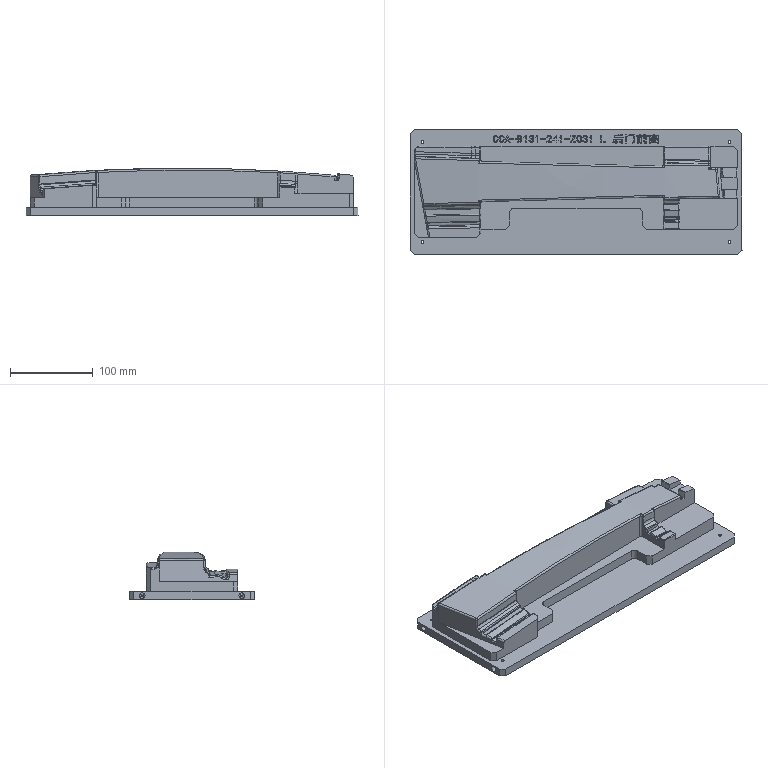NC program | NX | posted with a generic post | part box 400 x 150 x 57.494 mm
Lines 1 to 1105 of 16235:
N10 G17 G21 G94 G90
(B1 , TOOL : D16)
N12 T00 M6
N14 G54
N16 G17 G0 G90 X0. Y-75.996 S2500 M3
N18 G43 Z70.002 H0
N20 Z61.781
N22 G94 G1 Z61.481 F3000.
N24 Y-60.796
N26 X-199.991
N28 G2 X-200.795 Y-59.991 R0.804
N30 G1 Y60.124
N32 G2 X-199.989 Y60.931 R0.806
N34 G1 X199.992
N36 G2 X200.795 Y60.128 R0.803
N38 G1 X200.796 Y-59.991
N40 G2 X199.991 Y-60.796 R0.805
N42 G1 X0.
N44 Y-52.796
N46 X-192.795
N48 Y52.931
N50 X192.795
N52 X192.796 Y-52.796
N54 X0.
N56 Y-44.796
N58 X-184.795
N60 Y44.931
N62 X184.795
N64 X184.796 Y-44.796
N66 X0.
N68 Y-36.796
N70 X-176.795
N72 Y36.931
N74 X176.795
N76 X176.796 Y-36.796
N78 X0.
N80 Y-28.796
N82 X-168.795
N84 Y28.931
N86 X168.795
N88 X168.796 Y-28.796
N90 X0.
N92 Y-20.796
N94 X-160.795
N96 Y20.931
N98 X160.795
N100 X160.796 Y-20.796
N102 X0.
N104 Y-12.796
N106 X-152.795
N108 Y12.931
N110 X152.795
N112 X152.796 Y-12.796
N114 X0.
N116 Y-4.796
N118 X-144.795
N120 Y4.931
N122 X144.796
N124 Y-4.796
N126 X0.
N128 X-7.995 Z61.76
N130 Z62.06
N132 G0 Z62.753
N134 X0. Y-75.996
N136 Z60.809
N138 G1 Z60.509
N140 Y-60.796
N142 X-199.991
N144 G2 X-200.795 Y-59.991 R0.804
N146 G1 Y60.124
N148 G2 X-199.989 Y60.931 R0.807
N150 G1 X199.992
N152 G2 X200.795 Y60.128 R0.803
N154 G1 X200.796 Y-59.991
N156 G2 X199.991 Y-60.796 R0.805
N158 G1 X0.
N160 Y-52.796
N162 X-192.795
N164 Y52.931
N166 X192.795
N168 X192.796 Y-52.796
N170 X0.
N172 Y-44.796
N174 X-184.795
N176 Y44.931
N178 X184.795
N180 X184.796 Y-44.796
N182 X0.
N184 Y-36.796
N186 X-176.795
N188 Y36.931
N190 X176.796
N192 Y-36.796
N194 X0.
N196 Y-28.796
N198 X-168.795
N200 Y28.931
N202 X168.796
N204 Y-28.796
N206 X0.
N208 Y-20.796
N210 X-160.795
N212 Y20.931
N214 X160.796
N216 Y-20.796
N218 X0.
N220 Y-12.796
N222 X-152.795
N224 Y12.931
N226 X152.796
N228 Y-12.796
N230 X0.
N232 Y-4.796
N234 X-144.795
N236 Y4.931
N238 X144.796
N240 Y-4.796
N242 X0.
N244 X-7.995 Z60.788
N246 Z61.088
N248 G0 Z61.781
N250 X0. Y-75.996
N252 Z59.837
N254 G1 Z59.537
N256 Y-60.796
N258 X-199.991
N260 G2 X-200.796 Y-59.991 R0.805
N262 G1 Y60.124
N264 G2 X-199.989 Y60.931 R0.807
N266 G1 X199.992
N268 G2 X200.796 Y60.127 R0.803
N270 G1 Y-59.991
N272 G2 X199.991 Y-60.796 R0.805
N274 G1 X0.
N276 Y-52.796
N278 X-192.796
N280 Y52.931
N282 X192.796
N284 Y-52.796
N286 X0.
N288 Y-44.796
N290 X-184.796
N292 Y44.931
N294 X184.796
N296 Y-44.796
N298 X0.
N300 Y-36.796
N302 X-176.796
N304 Y36.931
N306 X176.796
N308 Y-36.796
N310 X0.
N312 Y-28.796
N314 X-168.796
N316 Y28.931
N318 X168.796
N320 Y-28.796
N322 X0.
N324 Y-20.796
N326 X-160.796
N328 Y20.931
N330 X160.796
N332 Y-20.796
N334 X0.
N336 Y-12.796
N338 X-152.796
N340 Y12.931
N342 X152.796
N344 Y-12.796
N346 X0.
N348 Y-4.796
N350 X-144.796
N352 Y4.931
N354 X144.796
N356 Y-4.796
N358 X0.
N360 X-7.995 Z59.816
N362 Z60.116
N364 G0 Z60.809
N366 X0. Y-75.996
N368 Z58.865
N370 G1 Z58.565
N372 Y-60.796
N374 X-199.991
N376 G2 X-200.796 Y-59.991 R0.805
N378 G1 Y60.124
N380 G2 X-199.989 Y60.931 R0.807
N382 G1 X199.992
N384 G2 X200.796 Y60.127 R0.803
N386 G1 Y-59.991
N388 G2 X199.991 Y-60.796 R0.805
N390 G1 X0.
N392 Y-52.796
N394 X-192.796
N396 Y52.931
N398 X192.796
N400 Y-52.796
N402 X0.
N404 Y-44.796
N406 X-184.796
N408 Y44.931
N410 X184.796
N412 Y-44.796
N414 X0.
N416 Y-36.796
N418 X-176.796
N420 Y36.931
N422 X176.796
N424 Y-36.796
N426 X0.
N428 Y-28.796
N430 X-168.796
N432 Y28.931
N434 X168.796
N436 Y-28.796
N438 X0.
N440 Y-20.796
N442 X-160.796
N444 Y20.931
N446 X160.796
N448 Y-20.796
N450 X0.
N452 Y-12.796
N454 X-152.796
N456 Y12.931
N458 X152.796
N460 Y-12.796
N462 X0.
N464 Y-4.796
N466 X-144.796
N468 Y4.931
N470 X144.796
N472 Y-4.796
N474 X0.
N476 X-7.995 Z58.844
N478 Z59.144
N480 G0 Z59.837
N482 X87.927 Y-75.996
N484 Z57.893
N486 G1 Z57.593
N488 Y-60.796
N490 X-199.991
N492 G2 X-200.796 Y-59.991 R0.805
N494 G1 Y60.124
N496 G2 X-199.988 Y60.931 R0.807
N498 G1 X199.992
N500 G2 X200.796 Y60.127 R0.804
N502 G1 Y-59.991
N504 G2 X199.991 Y-60.796 R0.805
N506 G1 X87.927
N508 Y-52.796
N510 X-192.796
N512 Y52.931
N514 X192.796
N516 Y-52.796
N518 X87.927
N520 Y-44.796
N522 X-184.796
N524 Y44.931
N526 X184.796
N528 Y-44.796
N530 X87.927
N532 Y-36.796
N534 X-176.796
N536 Y36.931
N538 X-42.086
N540 G3 X-41.693 Y29.269 R9.056
N542 X16.045 Y25.973 R33.831
N544 X16.171 Y36.931 R9.881
N546 G1 X14.83 Y36.059
N548 G2 X14.727 Y26.88 R8.281
N550 X-40.28 Y30.02 R32.231
N552 X-33.916 Y40.973 R7.456
N554 X8.586 Y39.798 R373.335
N556 X14.83 Y36.059 R8.281
N558 G1 X16.171 Y36.931
N560 X176.796
N562 Y-36.796
N564 X87.927
N566 Y-28.796
N568 X-168.796
N570 Y28.931
N572 X-50.124
N574 G3 X-48.756 Y25.513 R17.056
N576 X22.644 Y21.449 R41.831
N578 X25.575 Y28.931 R17.881
N580 G1 X168.796
N582 Y-28.796
N584 X87.927
N586 Y-20.796
N588 X-160.796
N590 Y20.931
N592 X-55.371
N594 G3 X29.241 Y16.924 R49.831
N596 X31.49 Y20.931 R25.881
N598 G1 X160.796
N600 Y-20.796
N602 X87.927
N604 Y-12.796
N606 X-152.796
N608 Y12.931
N610 X-59.845
N612 G3 X-49.493 Y1.274 R57.831
N614 G1 X-54.704 Y-4.796
N616 X-144.796
N618 Y4.931
N620 X-63.937
N622 G3 X-54.704 Y-4.796 R65.831
N624 G1 X-49.493 Y1.274
N626 G3 X35.837 Y12.398 R57.831
N628 X36.195 Y12.931 R33.881
N630 G1 X152.796
N632 Y-12.796
N634 X87.927
N636 Y-4.796
N638 X31.058
N640 G3 X40.291 Y4.931 R65.831
N642 G1 X144.796
N644 Y-4.796
N646 X87.927
N648 X79.932 Z57.872
N650 Z58.172
N652 G0 Z58.865
N654 X115.754 Y-75.996
N656 Z56.921
N658 G1 Z56.621
N660 Y-60.796
N662 X-199.991
N664 G2 X-200.796 Y-59.991 R0.805
N666 G1 Y60.123
N668 G2 X-199.988 Y60.931 R0.807
N670 G1 X199.992
N672 G2 X200.796 Y60.127 R0.804
N674 G1 Y-59.991
N676 G2 X199.991 Y-60.796 R0.805
N678 G1 X115.754
N680 Y-52.796
N682 X-192.796
N684 Y52.931
N686 X192.796
N688 Y-52.796
N690 X115.754
N692 Y-44.796
N694 X-184.796
N696 Y44.931
N698 X184.796
N700 Y-44.796
N702 X115.754
N704 Y-36.796
N706 X-176.796
N708 Y36.931
N710 X-86.652
N712 G3 X-86.764 Y30.88 R10.157
N714 G1 X-86.484 Y29.921
N716 X-86.44 Y29.791
N718 X-73.208 Y-4.362
N720 X-73.191 Y-4.404
N722 X-70.007 Y-11.971
N724 G3 X-62.361 Y-18.05 R10.172
N726 X-54.259 Y-18.809 R52.591
N728 G1 X-47.895 Y-18.91
N730 G3 X0.89 Y-18.142 R1369.321
N732 G1 X1.866 Y-18.098
N734 G3 X38.689 Y-16.323 R773.769
N736 G1 X38.754 Y-16.317
N738 X43.056 Y-15.829
N740 G3 X50.776 Y-12.317 R13.728
N742 X51.025 Y-12.028 R1.6
N744 G1 X52.351 Y-10.052
N746 G3 X52.576 Y-9.544 R1.6
N748 G1 X61.809 Y27.818
N750 G3 X59.692 Y36.931 R10.318
N752 G1 X58.467 Y35.902
N754 G2 X60.256 Y28.202 R8.718
N756 G1 X51.023 Y-9.16
N758 X49.696 Y-11.137
N760 G2 X42.876 Y-14.24 R12.128
N762 G1 X38.574 Y-14.727
N764 G2 X1.811 Y-16.499 R772.169
N766 G1 X0.817 Y-16.544
N768 G2 X-47.87 Y-17.31 R1367.721
N770 G1 X-54.233 Y-17.209
N772 G2 X-62.089 Y-16.473 R50.991
N774 X-68.533 Y-11.35 R8.572
N776 G1 X-71.716 Y-3.784
N778 X-84.948 Y30.369
N780 X-85.228 Y31.329
N782 G2 X-77.868 Y42.241 R8.557
N784 G1 X-74.697 Y42.559
N786 G2 X-51.844 Y42.963 R431.979
N788 X30.652 Y40.733 R2438.287
N790 X52.806 Y38.952 R306.533
N792 X58.467 Y35.902 R8.718
N794 G1 X59.692 Y36.931
N796 X176.796
N798 Y-36.796
N800 X115.754
N802 Y-28.796
N804 X-168.796
N806 Y28.931
N808 X-94.526
N810 G3 X-94.443 Y28.638 R18.157
N812 G1 X-94.163 Y27.679
N814 G3 X-93.9 Y26.901 R9.6
N816 G1 X-80.647 Y-7.305
N818 X-80.587 Y-7.454
N820 X-77.381 Y-15.073
N822 G3 X-76.493 Y-16.893 R18.172
N824 G1 X-83.476 Y-20.796
N826 X-160.796
N828 Y20.931
N830 X-100.166
N832 X-88.086 Y-10.249
N834 X-87.983 Y-10.504
N836 X-84.755 Y-18.176
N838 G3 X-83.476 Y-20.796 R26.172
N840 G1 X-95.679 Y-12.796
N842 X-152.796
N844 Y12.931
N846 X-105.646
N848 X-95.679 Y-12.796
N850 X-107.358 Y-4.796
N852 X-144.796
N854 Y4.931
N856 X-111.126
N858 X-107.358 Y-4.796
N860 X-95.679 Y-12.796
N862 X-83.476 Y-20.796
N864 X-76.493 Y-16.893
N866 G3 X-63.721 Y-25.933 R18.172
N868 X-54.387 Y-26.808 R60.591
N870 G1 X-47.912 Y-26.91
N872 G3 X1.205 Y-26.136 R1377.321
N874 G1 X2.145 Y-26.093
N876 G3 X39.346 Y-24.297 R781.769
N878 G1 X39.574 Y-24.276
N880 X43.957 Y-23.779
N882 G3 X56.177 Y-18.219 R21.728
N884 X57.667 Y-16.487 R9.6
N886 G1 X58.994 Y-14.51
N888 G3 X60.343 Y-11.463 R9.6
N890 G1 X69.576 Y25.899
N892 G3 X70.06 Y28.931 R18.318
N894 G1 X168.796
N896 Y-28.796
N898 X115.754
N900 Y-20.796
N902 X64.41
N904 X65.636 Y-18.969
N906 G3 X68.109 Y-13.383 R17.6
N908 G1 X76.589 Y20.931
N910 X160.796
N912 Y-20.796
N914 X115.754
N916 Y-12.796
N918 X76.494
N920 X82.852 Y12.931
N922 X152.796
N924 Y-12.796
N926 X115.754
N928 Y-4.796
N930 X86.712
N932 X89.116 Y4.931
N934 X144.796
N936 Y-4.796
N938 X115.754
N940 X107.759 Z56.9
N942 Z57.2
N944 G0 Z57.893
N946 X133.513 Y-75.996
N948 Z55.949
N950 G1 Z55.649
N952 Y-60.796
N954 X-199.991
N956 G2 X-200.796 Y-59.991 R0.805
N958 G1 Y60.127
N960 G2 X-199.992 Y60.931 R0.804
N962 G1 X199.992
N964 G2 X200.796 Y60.127 R0.804
N966 G1 Y-59.991
N968 G2 X199.991 Y-60.796 R0.805
N970 G1 X133.513
N972 Y-52.796
N974 X-192.796
N976 Y52.931
N978 X192.796
N980 Y-52.796
N982 X133.513
N984 Y-44.796
N986 X-184.796
N988 Y44.931
N990 X-98.572
N992 G3 X-102.445 Y44.559 R147.846
N994 X-111.458 Y32.044 R10.375
N996 G1 X-111.422 Y31.894
N998 X-98.613 Y-11.586
N1000 G3 X-89.808 Y-19.099 R10.541
N1002 X-79.694 Y-19.872 R87.287
N1004 X-52.81 Y-19.909 R729.221
N1006 X-4.109 Y-18.828 R3701.209
N1008 X40.624 Y-17.401 R2928.451
N1010 X63.73 Y-16.097 R686.126
N1012 X73.666 Y-14.689 R74.514
N1014 X81.599 Y-6.236 R10.131
N1016 G1 X86.58 Y27.984
N1018 G3 X77.898 Y39.823 R10.466
N1020 X62.654 Y41.505 R150.989
N1022 X29.679 Y42.972 R1123.908
N1024 X-42.853 Y44.918 R9082.565
N1026 G1 X-43.202 Y44.931
N1028 X-43.263 Y43.332
N1030 X-42.902 Y43.318
N1032 G2 X29.632 Y41.372 R9080.965
N1034 X62.56 Y39.908 R1122.308
N1036 X77.641 Y38.243 R149.389
N1038 X84.996 Y28.214 R8.866
N1040 G1 X80.015 Y-6.006
N1042 G2 X73.336 Y-13.124 R8.531
N1044 X63.613 Y-14.501 R72.914
N1046 X40.561 Y-15.803 R684.526
N1048 X-4.151 Y-17.229 R2926.851
N1050 X-52.838 Y-18.309 R3699.609
N1052 X-79.665 Y-18.272 R727.621
N1054 X-89.601 Y-17.512 R85.687
N1056 X-97.077 Y-11.137 R8.941
N1058 G1 X-109.887 Y32.346
N1060 X-109.934 Y32.593
N1062 G2 X-102.271 Y42.969 R8.775
N1064 X-87.433 Y43.831 R146.246
N1066 X-58.148 Y43.644 R1072.441
N1068 G1 X-45.883 Y43.398
N1070 X-43.895 Y43.356
N1072 X-43.263 Y43.332
N1074 X-43.202 Y44.931
N1076 X184.796
N1078 Y-44.796
N1080 X133.513
N1082 Y-36.796
N1084 X-176.796
N1086 Y36.931
N1088 X-119.497
N1090 G3 X-119.291 Y30.414 R18.375
N1092 X-119.096 Y29.633 R9.6
N1094 G1 X-106.29 Y-13.836
N1096 G3 X-100.554 Y-22.721 R18.541
N1098 G1 X-105.759 Y-28.796
N1100 X-168.796
N1102 Y28.931
N1104 X-127.154
N1106 X-127.12 Y28.773
N1108 G3 X-126.77 Y27.372 R17.6
N1110 G1 X-113.966 Y-16.088
N1112 G3 X-105.759 Y-28.796 R26.541
N1114 G1 X-120.823 Y-20.796
N1116 X-160.796
N1118 Y20.931
N1120 X-133.212
N1122 X-121.642 Y-18.342
N1124 G3 X-120.823 Y-20.796 R34.541
N1126 G1 X-131.616 Y-12.796
N1128 X-152.796
N1130 Y12.931
N1132 X-139.195
N1134 X-131.616 Y-12.796
N1136 X-142.313 Y-4.796
N1138 X-144.796
N1140 Y3.633
N1142 X-142.313 Y-4.796
N1144 X-131.616 Y-12.796
N1146 X-120.823 Y-20.796
N1148 X-105.759 Y-28.796
N1150 X-100.554 Y-22.721
N1152 G3 X-90.848 Y-27.031 R18.541
N1154 X-79.846 Y-27.87 R95.287
N1156 X-52.68 Y-27.908 R737.221
N1158 X-3.897 Y-26.825 R3709.209
N1160 X40.94 Y-25.395 R2936.451
N1162 X64.315 Y-24.075 R694.126
N1164 X75.319 Y-22.517 R82.514
N1166 X89.515 Y-7.389 R18.131
N1168 G1 X94.496 Y26.831
N1170 G3 X93.124 Y36.931 R18.466
N1172 G1 X176.796
N1174 Y-36.796
N1176 X133.513
N1178 Y-28.796
N1180 X81.865
N1182 G3 X97.432 Y-8.541 R26.131
N1184 G1 X102.413 Y25.679
N1186 G3 X102.683 Y28.931 R26.466
N1188 G1 X168.796
N1190 Y-28.796
N1192 X133.513
N1194 Y-20.796
N1196 X101.712
N1198 G3 X105.348 Y-9.693 R34.131
N1200 G1 X109.806 Y20.931
N1202 X160.796
N1204 Y-20.796
N1206 X133.513
N1208 Y-12.796
N1210 X112.934
N1212 G3 X113.265 Y-10.846 R42.131
N1214 G1 X116.726 Y12.931
N1216 X152.796
N1218 Y-12.796
N1220 X133.513
N1222 Y-4.796
N1224 X122.23
N1226 X123.646 Y4.931
N1228 X144.796
N1230 Y-4.796
N1232 X133.513
N1234 X125.518 Z55.928
N1236 Z56.228
N1238 G0 Z56.921
N1240 X143.696 Y-75.996
N1242 Z54.977
N1244 G1 Z54.677
N1246 Y-60.796
N1248 X-199.991
N1250 G2 X-200.796 Y-59.991 R0.805
N1252 G1 Y60.127
N1254 G2 X-199.992 Y60.931 R0.804
N1256 G1 X199.992
N1258 G2 X200.796 Y60.127 R0.804
N1260 G1 Y-59.991
N1262 G2 X199.991 Y-60.796 R0.805
N1264 G1 X143.696
N1266 Y-52.796
N1268 X-192.796
N1270 Y52.931
N1272 X192.796
N1274 Y-52.796
N1276 X143.696
N1278 Y-44.796
N1280 X-184.796
N1282 Y44.931
N1284 X-128.023
N1286 G3 X-131.505 Y37.418 R12.003
N1288 X-131.485 Y37.006 R1.6
N1290 G1 X-131.133 Y35.03
N1292 X-131.109 Y34.919
N1294 X-119.29 Y-11.944
N1296 G3 X-111.874 Y-19.336 R10.183
N1298 X-104.708 Y-20.37 R36.091
N1300 X-82.63 Y-20.719 R408.12
N1302 G1 X-80.641 Y-20.701
N1304 G3 X-47.694 Y-20.07 R1976.768
N1306 G1 X31.152 Y-18.005
N1308 X31.157
N1310 X51.538 Y-17.404
N1312 X51.561 Y-17.403
N1314 X53.538 Y-17.316
N1316 G3 X77.868 Y-16.187 R778.745
N1318 X91.455 Y-14.824 R179.801
N1320 G1 X91.527 Y-14.812
N1322 X93.746 Y-14.4
N1324 G3 X101.847 Y-7.582 R10.729
N1326 G1 X102.155 Y-6.752
N1328 G3 X102.247 Y-6.353 R1.6
N1330 G1 X105.763 Y29.224
N1332 G3 X105.738 Y29.702 R1.6
N1334 G1 X105.131 Y32.667
N1336 G3 X105.007 Y33.037 R1.6
N1338 X95.981 Y39.665 R11.884
N1340 G1 X93.45 Y40.029
N1342 X93.408 Y40.035
N1344 G3 X75.416 Y41.526 R270.971
N1346 X46.565 Y42.632 R1197.361
N1348 G1 X-41.07 Y44.931
N1350 X-41.112 Y43.332
N1352 X46.523 Y41.033
N1354 G2 X75.337 Y39.928 R1195.761
N1356 X93.222 Y38.445 R269.371
N1358 G1 X95.753 Y38.081
N1360 G2 X103.564 Y32.346 R10.284
N1362 G1 X104.17 Y29.381
N1364 X100.655 Y-6.195
N1366 X100.347 Y-7.025
N1368 G2 X93.454 Y-12.827 R9.129
N1370 G1 X91.235 Y-13.239
N1372 G2 X77.769 Y-14.59 R178.201
N1374 X53.478 Y-15.717 R777.145
N1376 G1 X51.491 Y-15.804
N1378 X31.11 Y-16.406
N1380 X-47.738 Y-18.471
N1382 G2 X-80.659 Y-19.101 R1975.168
N1384 G1 X-82.646 Y-19.119
N1386 G2 X-104.64 Y-18.772 R406.52
N1388 X-111.488 Y-17.784 R34.491
N1390 X-117.739 Y-11.553 R8.583
N1392 G1 X-129.558 Y35.311
N1394 X-129.91 Y37.287
N1396 G2 X-119.409 Y46.839 R10.403
N1398 X-113.448 Y46.496 R11.733
N1400 X-110.158 Y44.37 R7.655
N1402 X-91.588 Y44.476 R505.279
N1404 X-66.748 Y44.004 R1624.628
N1406 G1 X-41.112 Y43.332
N1408 X-41.07 Y44.931
N1410 X184.796
N1412 Y-44.796
N1414 X143.696
N1416 Y-36.796
N1418 X-176.796
N1420 Y36.931
N1422 X-139.504
N1424 G3 X-139.361 Y35.602 R9.6
N1426 G1 X-139.009 Y33.625
N1428 G3 X-138.866 Y32.963 R9.6
N1430 G1 X-127.047 Y-13.901
N1432 G3 X-121.672 Y-22.887 R18.183
N1434 G1 X-127.064 Y-28.796
N1436 X-168.796
N1438 Y28.931
N1440 X-146.1
N1442 X-134.804 Y-15.857
N1444 G3 X-127.064 Y-28.796 R26.183
N1446 G1 X-141.663 Y-20.796
N1448 X-160.796
N1450 Y20.931
N1452 X-152.333
N1454 X-142.561 Y-17.814
N1456 G3 X-141.663 Y-20.796 R34.183
N1458 G1 X-152.077 Y-12.796
N1460 X-152.796
N1462 Y-9.946
N1464 X-152.077 Y-12.796
N1466 X-141.663 Y-20.796
N1468 X-127.064 Y-28.796
N1470 X-121.672 Y-22.887
N1472 G3 X-113.805 Y-27.1 R18.183
N1474 X-105.051 Y-28.363 R44.091
N1476 X-82.548 Y-28.719 R416.12
N1478 G1 X-80.562 Y-28.701
N1480 G3 X-47.48 Y-28.067 R1984.768
N1482 G1 X31.368 Y-26.003
N1484 X31.386 Y-26.002
N1486 X51.803 Y-25.399
N1488 X51.882 Y-25.396
N1490 X53.836 Y-25.311
N1492 G3 X78.364 Y-24.172 R786.745
N1494 X92.646 Y-22.735 R187.801
N1496 G1 X92.898 Y-22.694
N1498 X95.207 Y-22.265
N1500 G3 X109.348 Y-10.363 R18.729
N1502 G1 X109.656 Y-9.533
N1504 G3 X110.208 Y-7.14 R9.6
N1506 G1 X113.724 Y28.437
N1508 G3 X113.576 Y31.306 R9.6
N1510 G1 X112.969 Y34.27
N1512 G3 X112.221 Y36.494 R9.6
N1514 X112.005 Y36.931 R19.884
N1516 G1 X176.796
N1518 Y-36.796
N1520 X143.696
N1522 Y-28.796
N1524 X101.389
N1526 G3 X116.849 Y-13.145 R26.729
N1528 G1 X117.157 Y-12.315
N1530 G3 X118.169 Y-7.926 R17.6
N1532 G1 X121.685 Y27.65
N1534 G3 X121.765 Y28.931 R17.6
N1536 G1 X168.796
N1538 Y-28.796
N1540 X143.696
N1542 Y-20.796
N1544 X122.102
N1546 G3 X124.35 Y-15.926 R34.729
N1548 G1 X124.657 Y-15.096
N1550 G3 X126.131 Y-8.713 R25.6
N1552 G1 X129.06 Y20.931
N1554 X160.796
N1556 Y-20.796
N1558 X143.696
N1560 Y-12.796
N1562 X133.6
N1564 G3 X134.092 Y-9.5 R33.6
N1566 G1 X136.308 Y12.931
N1568 X152.796
N1570 Y-12.796
N1572 X143.696
N1574 Y-4.796
N1576 X142.596
N1578 X143.557 Y4.931
N1580 X144.796
N1582 Y-4.796
N1584 X143.696
N1586 X135.701 Z54.956
N1588 Z55.256
N1590 G0 Z55.949
N1592 X215.996 Y-0.369
N1594 Z54.005
N1596 G1 Z53.705
N1598 X200.796
N1600 Y-59.991
N1602 G2 X199.991 Y-60.796 R0.806
N1604 G1 X-199.991
N1606 G2 X-200.796 Y-59.991 R0.805
N1608 G1 Y60.127
N1610 G2 X-199.992 Y60.931 R0.804
N1612 G1 X199.992
N1614 G2 X200.796 Y60.127 R0.804
N1616 G1 Y-0.369
N1618 X192.796
N1620 Y-52.796
N1622 X-192.796
N1624 Y52.931
N1626 X192.796
N1628 Y-0.369
N1630 X184.796
N1632 Y-44.796
N1634 X-184.796
N1636 Y44.931
N1638 X-145.142
N1640 G3 X-147.406 Y35.942 R10.431
N1642 G1 X-136.539 Y-11.494
N1644 X-136.535 Y-11.508
N1646 X-135.761 Y-14.752
N1648 G3 X-127.39 Y-22.725 R10.621
N1650 X-116.316 Y-23.773 R61.036
N1652 X-109.461 Y-21.28 R10.582
N1654 G1 X-106.836 Y-21.3
N1656 G3 X-81.016 Y-20.943 R1035.477
N1658 G1 X-33.917 Y-19.71
N1660 X-32.924 Y-19.684
N1662 X-31.778 Y-19.654
N1664 X10.795 Y-18.539
N1666 X11.788 Y-18.513
N1668 X12.783 Y-18.487
N1670 X19.737 Y-18.305
N1672 X23.712 Y-18.201
N1674 X24.706 Y-18.175
N1676 X64.578 Y-17.131
N1678 G3 X85.832 Y-16.368 R1228.651
N1680 X100.187 Y-15.437 R354.557
N1682 G1 X100.221 Y-15.458
N1684 X102.311 Y-16.764
N1686 G3 X102.604 Y-16.907 R1.6
N1688 X118.847 Y-9.766 R12.77
N1690 X118.934 Y-9.481 R1.6
N1692 G1 X119.136 Y-8.492
N1694 G3 X119.164 Y-8.293 R1.6
N1696 G1 X122.172 Y31.442
N1698 G3 X115.319 Y41.81 R10.141
N1700 X108.318 Y43.339 R31.968
N1702 X99.733 Y40.686 R11.033
N1704 G1 X94.324 Y41.052
N1706 G3 X70.41 Y42.013 R808.053
N1708 G1 X-41.027 Y44.931
N1710 X-41.069 Y43.332
N1712 X70.369 Y40.413
N1714 G2 X94.216 Y39.456 R806.453
N1716 G1 X100.318 Y39.043
N1718 G2 X108.14 Y41.748 R9.433
N1720 X114.805 Y40.295 R30.368
N1722 X120.576 Y31.563 R8.541
N1724 G1 X117.569 Y-8.172
N1726 X117.367 Y-9.16
N1728 G2 X103.158 Y-15.406 R11.17
N1730 G1 X101.068 Y-14.101
N1732 X100.69 Y-13.787
N1734 G2 X85.761 Y-14.77 R352.957
N1736 X64.536 Y-15.531 R1227.05
N1738 G1 X24.663 Y-16.575
N1740 X23.67 Y-16.602
N1742 X19.695 Y-16.705
N1744 X12.74 Y-16.887
N1746 X11.747 Y-16.914
N1748 X10.753 Y-16.939
N1750 X-31.82 Y-18.054
N1752 X-32.966 Y-18.085
N1754 X-33.959 Y-18.11
N1756 X-81.059 Y-19.344
N1758 G2 X-106.824 Y-19.7 R1033.877
N1760 G1 X-110.068 Y-19.675
N1762 G2 X-116.311 Y-22.173 R8.982
N1764 X-127.095 Y-21.153 R59.436
N1766 X-134.205 Y-14.381 R9.021
N1768 G1 X-134.979 Y-11.137
N1770 X-145.846 Y36.299
N1772 X-145.892 Y36.549
N1774 G2 X-138.648 Y46.868 R8.831
N1776 X-129.577 Y47.786 R72.492
N1778 X-115.435 Y47.989 R301.609
N1780 X-109.221 Y45.007 R9.46
N1782 G1 X-106.492 Y44.971
N1784 X-94.569 Y44.733
N1786 X-41.069 Y43.332
N1788 X-41.027 Y44.931
N1790 X184.796
N1792 Y-0.369
N1794 X176.796
N1796 Y-36.796
N1798 X-176.796
N1800 Y36.931
N1802 X-155.603
N1804 G3 X-155.214 Y34.2 R18.431
N1806 G1 X-144.332 Y-13.298
N1808 X-144.321 Y-13.347
N1810 X-143.543 Y-16.609
N1812 G3 X-140.038 Y-23.835 R18.621
N1814 G1 X-146.314 Y-28.796
N1816 X-168.796
N1818 Y28.931
N1820 X-162.214
N1822 X-152.126 Y-15.102
N1824 X-152.107 Y-15.186
N1826 X-151.324 Y-18.466
N1828 G3 X-146.314 Y-28.796 R26.621
N1830 G1 X-158.989 Y-20.796
N1832 X-160.796
N1834 Y-13.084
N1836 X-159.92 Y-16.906
N1838 X-159.892 Y-17.026
N1840 X-159.106 Y-20.323
N1842 G3 X-158.989 Y-20.796 R34.621
N1844 G1 X-146.314 Y-28.796
N1846 X-140.038 Y-23.835
N1848 G3 X-128.866 Y-30.588 R18.621
N1850 X-116.34 Y-31.773 R69.036
N1852 X-107.019 Y-29.299 R18.582
N1854 G1 X-106.861 Y-29.3
N1856 G3 X-80.806 Y-28.94 R1043.477
N1858 G1 X-33.709 Y-27.707
N1860 X-32.715 Y-27.681
N1862 X-31.566 Y-27.651
N1864 X11.003 Y-26.536
N1866 X11.997 Y-26.511
N1868 X12.994 Y-26.484
N1870 X19.947 Y-26.302
N1872 X23.922 Y-26.198
N1874 X24.918 Y-26.172
N1876 X64.795 Y-25.128
N1878 G3 X86.188 Y-24.36 R1236.651
N1880 X98.198 Y-23.626 R362.557
N1882 X99.831 Y-24.411 R9.6
N1884 X126.251 Y-12.797 R20.77
N1886 X126.772 Y-11.083 R9.6
N1888 G1 X126.974 Y-10.094
N1890 G3 X127.141 Y-8.896 R9.6
N1892 G1 X130.149 Y30.838
N1894 G3 X129.575 Y36.931 R18.141
N1896 G1 X176.796
N1898 Y-0.369
N1900 X168.796
N1902 Y-28.796
N1904 X123.093
N1906 G3 X133.655 Y-15.827 R28.77
N1908 X134.61 Y-12.685 R17.6
N1910 G1 X134.812 Y-11.696
N1912 G3 X135.118 Y-9.5 R17.6
N1914 G1 X138.027 Y28.931
N1916 X168.796
N1918 Y-0.369
N1920 X160.796
N1922 Y-20.796
N1924 X140.199
N1926 G3 X141.059 Y-18.857 R36.77
N1928 X142.448 Y-14.287 R25.6
N1930 G1 X142.65 Y-13.298
N1932 G3 X143.096 Y-10.104 R25.6
N1934 G1 X145.445 Y20.931
N1936 X160.796
N1938 Y-0.369
N1940 X152.796
N1942 Y-12.796
N1944 X150.849
N1946 G3 X151.073 Y-10.708 R33.6
N1948 G1 X152.796 Y12.059
N1950 Y-0.369
N1952 Y-8.364 Z53.984
N1954 Z54.284
N1956 G0 Z54.977
N1958 X215.996 Y0.068
N1960 Z53.033
N1962 G1 Z52.733
N1964 X200.796
N1966 Y-59.991
N1968 G2 X199.991 Y-60.796 R0.806
N1970 G1 X-199.991
N1972 G2 X-200.796 Y-59.991 R0.805
N1974 G1 Y60.127
N1976 G2 X-199.992 Y60.931 R0.804
N1978 G1 X199.992
N1980 G2 X200.796 Y60.127 R0.804
N1982 G1 Y0.068
N1984 X192.796
N1986 Y-52.796
N1988 X-192.796
N1990 Y52.931
N1992 X192.796
N1994 Y0.068
N1996 X184.796
N1998 Y-44.796
N2000 X-184.796
N2002 Y44.931
N2004 X-159.73
N2006 G3 X-161.799 Y37.11 R10.462
N2008 G1 X-161.732 Y36.626
N2010 X-161.712 Y36.515
N2012 X-150.903 Y-14.433
N2014 X-150.899 Y-14.45
N2016 X-150.81 Y-14.851
N2018 G3 X-142.255 Y-23.129 R10.822
N2020 X-133.385 Y-24.124 R59.621
N2022 X-116.004 Y-24.446 R336.373
N2024 X-108.719 Y-21.646 R11.091
N2026 G1 X-103.346 Y-21.528
N2028 X-103.339
N2030 X48.552 Y-17.551
N2032 X49.545 Y-17.525
N2034 X50.54 Y-17.499
N2036 X57.494 Y-17.316
N2038 X60.475 Y-17.239
N2040 X61.469 Y-17.212
N2042 X86.861 Y-16.547
N2044 G3 X98.873 Y-16.133 R1072.985
N2046 X106.582 Y-18.874 R10.885
N2048 X123.268 Y-17.258 R158.973
N2050 G1 X123.328 Y-17.248
N2052 X124.319 Y-17.06
N2054 G3 X133.484 Y-9.352 R12.151
N2056 G1 X134.056 Y-7.71
N2058 G3 X134.142 Y-7.279 R1.6
N2060 G1 X136.504 Y32.25
N2062 G3 X136.498 Y32.514 R1.6
N2064 X129.39 Y41.622 R10.392
N2066 X122.198 Y43.137 R32.954
N2068 X107.585 Y44.263 R252.829
N2070 X99.026 Y41.209 R11.893
N2072 G1 X90.293 Y41.492
N2074 X90.283 Y41.493
N2076 X-41.034 Y44.931
N2078 X-41.076 Y43.332
N2080 X90.241 Y39.893
N2082 X99.647 Y39.588
N2084 G2 X107.508 Y42.665 R10.293
N2086 X122.037 Y41.545 R251.229
N2088 X128.888 Y40.103 R31.354
N2090 X134.871 Y32.682 R8.792
N2092 G1 X134.906 Y32.346
N2094 X132.545 Y-7.184
N2096 X131.973 Y-8.826
N2098 G2 X124.024 Y-15.488 R10.551
N2100 G1 X123.03 Y-15.676
N2102 G2 X106.512 Y-17.275 R157.373
N2104 X99.484 Y-14.507 R9.285
N2106 X86.819 Y-14.948 R1071.385
N2108 G1 X61.427 Y-15.613
N2110 X60.433 Y-15.639
N2112 X57.452 Y-15.717
N2114 X50.497 Y-15.899
N2116 X49.504 Y-15.926
N2118 X48.51 Y-15.951
N2120 X-103.381 Y-19.929
N2122 X-109.369 Y-20.06
N2124 G2 X-116.016 Y-22.846 R9.491
N2126 X-133.32 Y-22.525 R334.773
N2128 X-141.958 Y-21.557 R58.021
N2130 X-149.248 Y-14.502 R9.222
N2132 G1 X-149.338 Y-14.101
N2134 X-160.147 Y36.847
N2136 X-160.214 Y37.33
N2138 G2 X-153.159 Y47.246 R8.862
N2140 G1 X-151.205 Y47.633
N2142 G2 X-138.288 Y48.421 R125.069
N2144 X-115.69 Y48.23 R534.23
N2146 X-108.955 Y45.109 R9.435
N2148 G1 X-41.076 Y43.332
N2150 X-41.034 Y44.931
N2152 X184.796
N2154 Y0.068
N2156 X176.796 Y0.067
N2158 Y-36.796
N2160 X-176.796
N2162 Y36.931
N2164 X-169.828
N2166 G3 X-169.723 Y36.006 R18.462
N2168 G1 X-169.655 Y35.523
N2170 G3 X-169.538 Y34.854 R9.6
N2172 G1 X-158.724 Y-16.114
N2174 X-158.712 Y-16.171
N2176 G3 X-155.199 Y-23.934 R18.822
N2178 G1 X-161.552 Y-28.796
N2180 X-168.796
N2182 Y-7.189
N2184 X-166.546 Y-17.795
N2186 G3 X-161.552 Y-28.796 R26.822
N2188 G1 X-155.199 Y-23.934
N2190 G3 X-143.739 Y-30.991 R18.822
N2192 X-133.71 Y-32.118 R67.621
N2194 X-115.945 Y-32.445 R344.373
N2196 X-106.04 Y-29.589 R19.091
N2198 G1 X-103.161 Y-29.526
N2200 X-103.138 Y-29.525
N2202 X48.76 Y-25.548
N2204 X49.754 Y-25.522
N2206 X50.751 Y-25.496
N2208 X57.704 Y-25.314